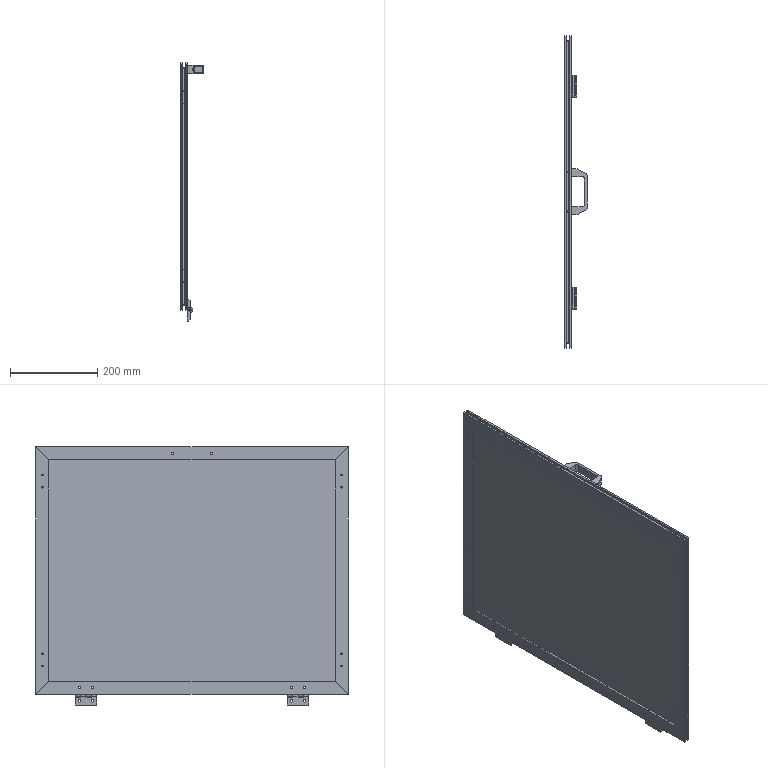Part | SolidWorks | 12 solids | 404 faces | box 51 x 717 x 593 mm | volume 2782623 mm3 | plane 216 | cylinder 144 | cone 44 | commonest cylinder face diameters 5 x44 3.3 x32 5.8 x20 6.4 x16 10 x12 16.345 x8